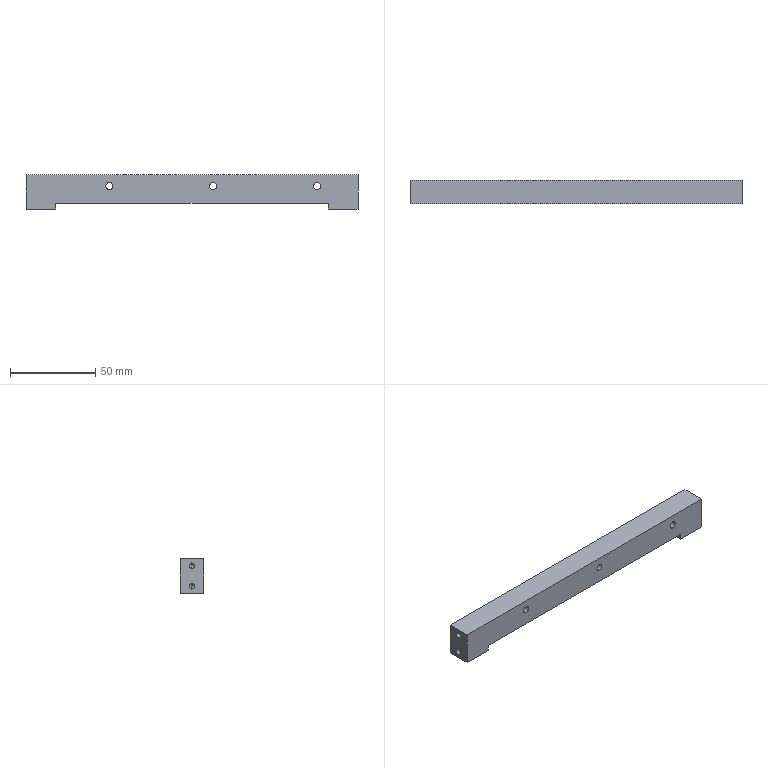Part | SolidWorks | features HoleWzd 3, ICE 2, ExtruThin 1 | 1 solid | 41 faces | box 195 x 14 x 20 mm | volume 45399 mm3 | cylinder 20 | plane 13 | cone 8 | commonest cylinder face diameters 3.3 x8 4.2 x6 8.8 x6
STEP:
#1=CARTESIAN_POINT('',(-19.6,11.,3.5));
#2=VERTEX_POINT('',#1);
#3=CARTESIAN_POINT('',(-28.4,11.,3.5));
#4=VERTEX_POINT('',#3);
#5=CARTESIAN_POINT('',(-24.,11.,3.5));
#6=DIRECTION('',(0.,1.,0.));
#7=DIRECTION('',(-1.,0.,0.));
#8=AXIS2_PLACEMENT_3D('',#5,#6,#7);
#9=CIRCLE('',#8,4.4);
#10=EDGE_CURVE('',#2,#4,#9,.T.);
#11=ORIENTED_EDGE('',*,*,#10,.F.);
#12=CARTESIAN_POINT('',(-19.6,14.,3.5));
#13=VERTEX_POINT('',#12);
#14=CARTESIAN_POINT('',(-19.6,11.,3.5));
#15=DIRECTION('',(0.,1.,0.));
#16=VECTOR('',#15,1000.);
#17=LINE('',#14,#16);
#18=EDGE_CURVE('',#2,#13,#17,.T.);
#19=ORIENTED_EDGE('',*,*,#18,.T.);
#20=CARTESIAN_POINT('',(-28.4,14.,3.5));
#21=VERTEX_POINT('',#20);
#22=CARTESIAN_POINT('',(-24.,14.,3.5));
#23=DIRECTION('',(0.,1.,0.));
#24=DIRECTION('',(-1.,0.,0.));
#25=AXIS2_PLACEMENT_3D('',#22,#23,#24);
#26=CIRCLE('',#25,4.4);
#27=EDGE_CURVE('',#13,#21,#26,.T.);
#28=ORIENTED_EDGE('',*,*,#27,.T.);
#29=CARTESIAN_POINT('',(-28.4,11.,3.5));
#30=DIRECTION('',(0.,1.,0.));
#31=VECTOR('',#30,1000.);
#32=LINE('',#29,#31);
#33=EDGE_CURVE('',#4,#21,#32,.T.);
#34=ORIENTED_EDGE('',*,*,#33,.F.);
#35=EDGE_LOOP('',(#11,#19,#28,#34));
#36=FACE_OUTER_BOUND('',#35,.T.);
#37=CARTESIAN_POINT('',(-24.,11.,3.5));
#38=DIRECTION('',(0.,1.,0.));
#39=DIRECTION('',(-1.,0.,0.));
#40=AXIS2_PLACEMENT_3D('',#37,#38,#39);
#41=CYLINDRICAL_SURFACE('',#40,4.4);
#42=ADVANCED_FACE('',(#36),#41,.F.);
#43=CARTESIAN_POINT('',(-80.6,11.,3.5));
#44=VERTEX_POINT('',#43);
#45=CARTESIAN_POINT('',(-89.4,11.,3.5));
#46=VERTEX_POINT('',#45);
#47=CARTESIAN_POINT('',(-85.,11.,3.5));
#48=DIRECTION('',(0.,1.,0.));
#49=DIRECTION('',(-1.,0.,0.));
#50=AXIS2_PLACEMENT_3D('',#47,#48,#49);
#51=CIRCLE('',#50,4.4);
#52=EDGE_CURVE('',#44,#46,#51,.T.);
#53=ORIENTED_EDGE('',*,*,#52,.F.);
#54=CARTESIAN_POINT('',(-80.6,14.,3.5));
#55=VERTEX_POINT('',#54);
#56=CARTESIAN_POINT('',(-80.6,11.,3.5));
#57=DIRECTION('',(0.,1.,0.));
#58=VECTOR('',#57,1000.);
#59=LINE('',#56,#58);
#60=EDGE_CURVE('',#44,#55,#59,.T.);
#61=ORIENTED_EDGE('',*,*,#60,.T.);
#62=CARTESIAN_POINT('',(-89.4,14.,3.5));
#63=VERTEX_POINT('',#62);
#64=CARTESIAN_POINT('',(-85.,14.,3.5));
#65=DIRECTION('',(0.,1.,0.));
#66=DIRECTION('',(-1.,0.,0.));
#67=AXIS2_PLACEMENT_3D('',#64,#65,#66);
#68=CIRCLE('',#67,4.4);
#69=EDGE_CURVE('',#55,#63,#68,.T.);
#70=ORIENTED_EDGE('',*,*,#69,.T.);
#71=CARTESIAN_POINT('',(-89.4,11.,3.5));
#72=DIRECTION('',(0.,1.,0.));
#73=VECTOR('',#72,1000.);
#74=LINE('',#71,#73);
#75=EDGE_CURVE('',#46,#63,#74,.T.);
#76=ORIENTED_EDGE('',*,*,#75,.F.);
#77=EDGE_LOOP('',(#53,#61,#70,#76));
#78=FACE_OUTER_BOUND('',#77,.T.);
#79=CARTESIAN_POINT('',(-85.,11.,3.5));
#80=DIRECTION('',(0.,1.,0.));
#81=DIRECTION('',(-1.,0.,0.));
#82=AXIS2_PLACEMENT_3D('',#79,#80,#81);
#83=CYLINDRICAL_SURFACE('',#82,4.4);
#84=ADVANCED_FACE('',(#78),#83,.F.);
#85=CARTESIAN_POINT('',(-141.6,11.,3.5));
#86=VERTEX_POINT('',#85);
#87=CARTESIAN_POINT('',(-150.4,11.,3.5));
#88=VERTEX_POINT('',#87);
#89=CARTESIAN_POINT('',(-146.,11.,3.5));
#90=DIRECTION('',(0.,1.,0.));
#91=DIRECTION('',(-1.,0.,0.));
#92=AXIS2_PLACEMENT_3D('',#89,#90,#91);
#93=CIRCLE('',#92,4.4);
#94=EDGE_CURVE('',#86,#88,#93,.T.);
#95=ORIENTED_EDGE('',*,*,#94,.F.);
#96=CARTESIAN_POINT('',(-141.6,14.,3.5));
#97=VERTEX_POINT('',#96);
#98=CARTESIAN_POINT('',(-141.6,11.,3.5));
#99=DIRECTION('',(0.,1.,0.));
#100=VECTOR('',#99,1000.);
#101=LINE('',#98,#100);
#102=EDGE_CURVE('',#86,#97,#101,.T.);
#103=ORIENTED_EDGE('',*,*,#102,.T.);
#104=CARTESIAN_POINT('',(-150.4,14.,3.5));
#105=VERTEX_POINT('',#104);
#106=CARTESIAN_POINT('',(-146.,14.,3.5));
#107=DIRECTION('',(0.,1.,0.));
#108=DIRECTION('',(-1.,0.,0.));
#109=AXIS2_PLACEMENT_3D('',#106,#107,#108);
#110=CIRCLE('',#109,4.4);
#111=EDGE_CURVE('',#97,#105,#110,.T.);
#112=ORIENTED_EDGE('',*,*,#111,.T.);
#113=CARTESIAN_POINT('',(-150.4,11.,3.5));
#114=DIRECTION('',(0.,1.,0.));
#115=VECTOR('',#114,1000.);
#116=LINE('',#113,#115);
#117=EDGE_CURVE('',#88,#105,#116,.T.);
#118=ORIENTED_EDGE('',*,*,#117,.F.);
#119=EDGE_LOOP('',(#95,#103,#112,#118));
#120=FACE_OUTER_BOUND('',#119,.T.);
#121=CARTESIAN_POINT('',(-146.,11.,3.5));
#122=DIRECTION('',(0.,1.,0.));
#123=DIRECTION('',(-1.,0.,0.));
#124=AXIS2_PLACEMENT_3D('',#121,#122,#123);
#125=CYLINDRICAL_SURFACE('',#124,4.4);
#126=ADVANCED_FACE('',(#120),#125,.F.);
#127=CARTESIAN_POINT('',(-10.1,7.,7.65));
#128=VERTEX_POINT('',#127);
#129=CARTESIAN_POINT('',(-10.1,7.,4.35));
#130=VERTEX_POINT('',#129);
#131=CARTESIAN_POINT('',(-10.1,7.,6.));
#132=DIRECTION('',(1.,0.,0.));
#133=DIRECTION('',(0.,0.,-1.));
#134=AXIS2_PLACEMENT_3D('',#131,#132,#133);
#135=CIRCLE('',#134,1.65);
#136=EDGE_CURVE('',#128,#130,#135,.T.);
#137=ORIENTED_EDGE('',*,*,#136,.F.);
#138=CARTESIAN_POINT('',(0.,7.,7.65));
#139=VERTEX_POINT('',#138);
#140=CARTESIAN_POINT('',(0.,7.,7.65));
#141=DIRECTION('',(1.,0.,0.));
#142=VECTOR('',#141,1000.);
#143=LINE('',#140,#142);
#144=EDGE_CURVE('',#128,#139,#143,.T.);
#145=ORIENTED_EDGE('',*,*,#144,.T.);
#146=CARTESIAN_POINT('',(0.,7.,4.35));
#147=VERTEX_POINT('',#146);
#148=CARTESIAN_POINT('',(0.,7.,6.));
#149=DIRECTION('',(1.,0.,0.));
#150=DIRECTION('',(0.,0.,-1.));
#151=AXIS2_PLACEMENT_3D('',#148,#149,#150);
#152=CIRCLE('',#151,1.65);
#153=EDGE_CURVE('',#139,#147,#152,.T.);
#154=ORIENTED_EDGE('',*,*,#153,.T.);
#155=CARTESIAN_POINT('',(0.,7.,4.35));
#156=DIRECTION('',(1.,0.,0.));
#157=VECTOR('',#156,1000.);
#158=LINE('',#155,#157);
#159=EDGE_CURVE('',#130,#147,#158,.T.);
#160=ORIENTED_EDGE('',*,*,#159,.F.);
#161=EDGE_LOOP('',(#137,#145,#154,#160));
#162=FACE_OUTER_BOUND('',#161,.T.);
#163=CARTESIAN_POINT('',(0.,7.,6.));
#164=DIRECTION('',(1.,0.,0.));
#165=DIRECTION('',(0.,0.,-1.));
#166=AXIS2_PLACEMENT_3D('',#163,#164,#165);
#167=CYLINDRICAL_SURFACE('',#166,1.65);
#168=ADVANCED_FACE('',(#162),#167,.F.);
#169=CARTESIAN_POINT('',(-11.091,7.,6.));
#170=VERTEX_POINT('',#169);
#171=CARTESIAN_POINT('',(-10.1,7.,4.35));
#172=DIRECTION('',(0.515,0.,-0.8572));
#173=VECTOR('',#172,1000.);
#174=LINE('',#171,#173);
#175=EDGE_CURVE('',#170,#130,#174,.T.);
#176=ORIENTED_EDGE('',*,*,#175,.F.);
#177=CARTESIAN_POINT('',(-10.1,7.,7.65));
#178=DIRECTION('',(0.515,0.,0.8572));
#179=VECTOR('',#178,1000.);
#180=LINE('',#177,#179);
#181=EDGE_CURVE('',#170,#128,#180,.T.);
#182=ORIENTED_EDGE('',*,*,#181,.T.);
#183=ORIENTED_EDGE('',*,*,#136,.T.);
#184=EDGE_LOOP('',(#176,#182,#183));
#185=FACE_OUTER_BOUND('',#184,.T.);
#186=CARTESIAN_POINT('',(-10.1,7.,6.));
#187=DIRECTION('',(1.,0.,0.));
#188=DIRECTION('',(0.,0.,-1.));
#189=AXIS2_PLACEMENT_3D('',#186,#187,#188);
#190=CONICAL_SURFACE('',#189,1.65,1.03);
#191=ADVANCED_FACE('',(#185),#190,.F.);
#192=CARTESIAN_POINT('',(-10.1,7.,-4.35));
#193=VERTEX_POINT('',#192);
#194=CARTESIAN_POINT('',(-10.1,7.,-7.65));
#195=VERTEX_POINT('',#194);
#196=CARTESIAN_POINT('',(-10.1,7.,-6.));
#197=DIRECTION('',(1.,0.,0.));
#198=DIRECTION('',(0.,0.,-1.));
#199=AXIS2_PLACEMENT_3D('',#196,#197,#198);
#200=CIRCLE('',#199,1.65);
#201=EDGE_CURVE('',#193,#195,#200,.T.);
#202=ORIENTED_EDGE('',*,*,#201,.F.);
#203=CARTESIAN_POINT('',(0.,7.,-4.35));
#204=VERTEX_POINT('',#203);
#205=CARTESIAN_POINT('',(0.,7.,-4.35));
#206=DIRECTION('',(1.,0.,0.));
#207=VECTOR('',#206,1000.);
#208=LINE('',#205,#207);
#209=EDGE_CURVE('',#193,#204,#208,.T.);
#210=ORIENTED_EDGE('',*,*,#209,.T.);
#211=CARTESIAN_POINT('',(0.,7.,-7.65));
#212=VERTEX_POINT('',#211);
#213=CARTESIAN_POINT('',(0.,7.,-6.));
#214=DIRECTION('',(1.,0.,0.));
#215=DIRECTION('',(0.,0.,-1.));
#216=AXIS2_PLACEMENT_3D('',#213,#214,#215);
#217=CIRCLE('',#216,1.65);
#218=EDGE_CURVE('',#204,#212,#217,.T.);
#219=ORIENTED_EDGE('',*,*,#218,.T.);
#220=CARTESIAN_POINT('',(0.,7.,-7.65));
#221=DIRECTION('',(1.,0.,0.));
#222=VECTOR('',#221,1000.);
#223=LINE('',#220,#222);
#224=EDGE_CURVE('',#195,#212,#223,.T.);
#225=ORIENTED_EDGE('',*,*,#224,.F.);
#226=EDGE_LOOP('',(#202,#210,#219,#225));
#227=FACE_OUTER_BOUND('',#226,.T.);
#228=CARTESIAN_POINT('',(0.,7.,-6.));
#229=DIRECTION('',(1.,0.,0.));
#230=DIRECTION('',(0.,0.,-1.));
#231=AXIS2_PLACEMENT_3D('',#228,#229,#230);
#232=CYLINDRICAL_SURFACE('',#231,1.65);
#233=ADVANCED_FACE('',(#227),#232,.F.);
#234=CARTESIAN_POINT('',(-11.091,7.,-6.));
#235=VERTEX_POINT('',#234);
#236=CARTESIAN_POINT('',(-10.1,7.,-7.65));
#237=DIRECTION('',(0.515,0.,-0.8572));
#238=VECTOR('',#237,1000.);
#239=LINE('',#236,#238);
#240=EDGE_CURVE('',#235,#195,#239,.T.);
#241=ORIENTED_EDGE('',*,*,#240,.F.);
#242=CARTESIAN_POINT('',(-10.1,7.,-4.35));
#243=DIRECTION('',(0.515,0.,0.8572));
#244=VECTOR('',#243,1000.);
#245=LINE('',#242,#244);
#246=EDGE_CURVE('',#235,#193,#245,.T.);
#247=ORIENTED_EDGE('',*,*,#246,.T.);
#248=ORIENTED_EDGE('',*,*,#201,.T.);
#249=EDGE_LOOP('',(#241,#247,#248));
#250=FACE_OUTER_BOUND('',#249,.T.);
#251=CARTESIAN_POINT('',(-10.1,7.,-6.));
#252=DIRECTION('',(1.,0.,0.));
#253=DIRECTION('',(0.,0.,-1.));
#254=AXIS2_PLACEMENT_3D('',#251,#252,#253);
#255=CONICAL_SURFACE('',#254,1.65,1.03);
#256=ADVANCED_FACE('',(#250),#255,.F.);
#257=CARTESIAN_POINT('',(-184.9,7.,-7.65));
#258=VERTEX_POINT('',#257);
#259=CARTESIAN_POINT('',(-184.9,7.,-4.35));
#260=VERTEX_POINT('',#259);
#261=CARTESIAN_POINT('',(-184.9,7.,-6.));
#262=DIRECTION('',(-1.,0.,0.));
#263=DIRECTION('',(0.,0.,1.));
#264=AXIS2_PLACEMENT_3D('',#261,#262,#263);
#265=CIRCLE('',#264,1.65);
#266=EDGE_CURVE('',#258,#260,#265,.T.);
#267=ORIENTED_EDGE('',*,*,#266,.F.);
#268=CARTESIAN_POINT('',(-195.,7.,-7.65));
#269=VERTEX_POINT('',#268);
#270=CARTESIAN_POINT('',(-195.,7.,-7.65));
#271=DIRECTION('',(-1.,0.,0.));
#272=VECTOR('',#271,1000.);
#273=LINE('',#270,#272);
#274=EDGE_CURVE('',#258,#269,#273,.T.);
#275=ORIENTED_EDGE('',*,*,#274,.T.);
#276=CARTESIAN_POINT('',(-195.,7.,-4.35));
#277=VERTEX_POINT('',#276);
#278=CARTESIAN_POINT('',(-195.,7.,-6.));
#279=DIRECTION('',(-1.,0.,0.));
#280=DIRECTION('',(0.,0.,1.));
#281=AXIS2_PLACEMENT_3D('',#278,#279,#280);
#282=CIRCLE('',#281,1.65);
#283=EDGE_CURVE('',#269,#277,#282,.T.);
#284=ORIENTED_EDGE('',*,*,#283,.T.);
#285=CARTESIAN_POINT('',(-195.,7.,-4.35));
#286=DIRECTION('',(-1.,0.,0.));
#287=VECTOR('',#286,1000.);
#288=LINE('',#285,#287);
#289=EDGE_CURVE('',#260,#277,#288,.T.);
#290=ORIENTED_EDGE('',*,*,#289,.F.);
#291=EDGE_LOOP('',(#267,#275,#284,#290));
#292=FACE_OUTER_BOUND('',#291,.T.);
#293=CARTESIAN_POINT('',(-195.,7.,-6.));
#294=DIRECTION('',(-1.,0.,0.));
#295=DIRECTION('',(0.,0.,1.));
#296=AXIS2_PLACEMENT_3D('',#293,#294,#295);
#297=CYLINDRICAL_SURFACE('',#296,1.65);
#298=ADVANCED_FACE('',(#292),#297,.F.);
#299=CARTESIAN_POINT('',(-183.909,7.,-6.));
#300=VERTEX_POINT('',#299);
#301=CARTESIAN_POINT('',(-184.9,7.,-4.35));
#302=DIRECTION('',(-0.515,0.,0.8572));
#303=VECTOR('',#302,1000.);
#304=LINE('',#301,#303);
#305=EDGE_CURVE('',#300,#260,#304,.T.);
#306=ORIENTED_EDGE('',*,*,#305,.F.);
#307=CARTESIAN_POINT('',(-184.9,7.,-7.65));
#308=DIRECTION('',(-0.515,0.,-0.8572));
#309=VECTOR('',#308,1000.);
#310=LINE('',#307,#309);
#311=EDGE_CURVE('',#300,#258,#310,.T.);
#312=ORIENTED_EDGE('',*,*,#311,.T.);
#313=ORIENTED_EDGE('',*,*,#266,.T.);
#314=EDGE_LOOP('',(#306,#312,#313));
#315=FACE_OUTER_BOUND('',#314,.T.);
#316=CARTESIAN_POINT('',(-184.9,7.,-6.));
#317=DIRECTION('',(-1.,0.,0.));
#318=DIRECTION('',(0.,0.,1.));
#319=AXIS2_PLACEMENT_3D('',#316,#317,#318);
#320=CONICAL_SURFACE('',#319,1.65,1.03);
#321=ADVANCED_FACE('',(#315),#320,.F.);
#322=CARTESIAN_POINT('',(-184.9,7.,4.35));
#323=VERTEX_POINT('',#322);
#324=CARTESIAN_POINT('',(-184.9,7.,7.65));
#325=VERTEX_POINT('',#324);
#326=CARTESIAN_POINT('',(-184.9,7.,6.));
#327=DIRECTION('',(-1.,0.,0.));
#328=DIRECTION('',(0.,0.,1.));
#329=AXIS2_PLACEMENT_3D('',#326,#327,#328);
#330=CIRCLE('',#329,1.65);
#331=EDGE_CURVE('',#323,#325,#330,.T.);
#332=ORIENTED_EDGE('',*,*,#331,.F.);
#333=CARTESIAN_POINT('',(-195.,7.,4.35));
#334=VERTEX_POINT('',#333);
#335=CARTESIAN_POINT('',(-195.,7.,4.35));
#336=DIRECTION('',(-1.,0.,0.));
#337=VECTOR('',#336,1000.);
#338=LINE('',#335,#337);
#339=EDGE_CURVE('',#323,#334,#338,.T.);
#340=ORIENTED_EDGE('',*,*,#339,.T.);
#341=CARTESIAN_POINT('',(-195.,7.,7.65));
#342=VERTEX_POINT('',#341);
#343=CARTESIAN_POINT('',(-195.,7.,6.));
#344=DIRECTION('',(-1.,0.,0.));
#345=DIRECTION('',(0.,0.,1.));
#346=AXIS2_PLACEMENT_3D('',#343,#344,#345);
#347=CIRCLE('',#346,1.65);
#348=EDGE_CURVE('',#334,#342,#347,.T.);
#349=ORIENTED_EDGE('',*,*,#348,.T.);
#350=CARTESIAN_POINT('',(-195.,7.,7.65));
#351=DIRECTION('',(-1.,0.,0.));
#352=VECTOR('',#351,1000.);
#353=LINE('',#350,#352);
#354=EDGE_CURVE('',#325,#342,#353,.T.);
#355=ORIENTED_EDGE('',*,*,#354,.F.);
#356=EDGE_LOOP('',(#332,#340,#349,#355));
#357=FACE_OUTER_BOUND('',#356,.T.);
#358=CARTESIAN_POINT('',(-195.,7.,6.));
#359=DIRECTION('',(-1.,0.,0.));
#360=DIRECTION('',(0.,0.,1.));
#361=AXIS2_PLACEMENT_3D('',#358,#359,#360);
#362=CYLINDRICAL_SURFACE('',#361,1.65);
#363=ADVANCED_FACE('',(#357),#362,.F.);
#364=CARTESIAN_POINT('',(-183.909,7.,6.));
#365=VERTEX_POINT('',#364);
#366=CARTESIAN_POINT('',(-184.9,7.,7.65));
#367=DIRECTION('',(-0.515,0.,0.8572));
#368=VECTOR('',#367,1000.);
#369=LINE('',#366,#368);
#370=EDGE_CURVE('',#365,#325,#369,.T.);
#371=ORIENTED_EDGE('',*,*,#370,.F.);
#372=CARTESIAN_POINT('',(-184.9,7.,4.35));
#373=DIRECTION('',(-0.515,0.,-0.8572));
#374=VECTOR('',#373,1000.);
#375=LINE('',#372,#374);
#376=EDGE_CURVE('',#365,#323,#375,.T.);
#377=ORIENTED_EDGE('',*,*,#376,.T.);
#378=ORIENTED_EDGE('',*,*,#331,.T.);
#379=EDGE_LOOP('',(#371,#377,#378));
#380=FACE_OUTER_BOUND('',#379,.T.);
#381=CARTESIAN_POINT('',(-184.9,7.,6.));
#382=DIRECTION('',(-1.,0.,0.));
#383=DIRECTION('',(0.,0.,1.));
#384=AXIS2_PLACEMENT_3D('',#381,#382,#383);
#385=CONICAL_SURFACE('',#384,1.65,1.03);
#386=ADVANCED_FACE('',(#380),#385,.F.);
#387=CARTESIAN_POINT('',(-146.,0.,1.4));
#388=VERTEX_POINT('',#387);
#389=CARTESIAN_POINT('',(-146.,0.,5.6));
#390=VERTEX_POINT('',#389);
#391=CARTESIAN_POINT('',(-146.,0.,3.5));
#392=DIRECTION('',(0.,1.,0.));
#393=DIRECTION('',(0.,0.,1.));
#394=AXIS2_PLACEMENT_3D('',#391,#392,#393);
#395=CIRCLE('',#394,2.1);
#396=EDGE_CURVE('',#388,#390,#395,.T.);
#397=ORIENTED_EDGE('',*,*,#396,.F.);
#398=CARTESIAN_POINT('',(-146.,11.,1.4));
#399=VERTEX_POINT('',#398);
#400=CARTESIAN_POINT('',(-146.,14.,1.4));
#401=DIRECTION('',(0.,1.,0.));
#402=VECTOR('',#401,1000.);
#403=LINE('',#400,#402);
#404=EDGE_CURVE('',#388,#399,#403,.T.);
#405=ORIENTED_EDGE('',*,*,#404,.T.);
#406=CARTESIAN_POINT('',(-146.,11.,5.6));
#407=VERTEX_POINT('',#406);
#408=CARTESIAN_POINT('',(-146.,11.,3.5));
#409=DIRECTION('',(0.,-1.,0.));
#410=DIRECTION('',(-1.,0.,0.));
#411=AXIS2_PLACEMENT_3D('',#408,#409,#410);
#412=CIRCLE('',#411,2.1);
#413=EDGE_CURVE('',#407,#399,#412,.T.);
#414=ORIENTED_EDGE('',*,*,#413,.F.);
#415=CARTESIAN_POINT('',(-146.,14.,5.6));
#416=DIRECTION('',(0.,1.,0.));
#417=VECTOR('',#416,1000.);
#418=LINE('',#415,#417);
#419=EDGE_CURVE('',#390,#407,#418,.T.);
#420=ORIENTED_EDGE('',*,*,#419,.F.);
#421=EDGE_LOOP('',(#397,#405,#414,#420));
#422=FACE_OUTER_BOUND('',#421,.T.);
#423=CARTESIAN_POINT('',(-146.,14.,3.5));
#424=DIRECTION('',(0.,1.,0.));
#425=DIRECTION('',(0.,0.,1.));
#426=AXIS2_PLACEMENT_3D('',#423,#424,#425);
#427=CYLINDRICAL_SURFACE('',#426,2.1);
#428=ADVANCED_FACE('',(#422),#427,.F.);
#429=CARTESIAN_POINT('',(-85.,0.,1.4));
#430=VERTEX_POINT('',#429);
#431=CARTESIAN_POINT('',(-85.,0.,5.6));
#432=VERTEX_POINT('',#431);
#433=CARTESIAN_POINT('',(-85.,0.,3.5));
#434=DIRECTION('',(0.,1.,0.));
#435=DIRECTION('',(0.,0.,1.));
#436=AXIS2_PLACEMENT_3D('',#433,#434,#435);
#437=CIRCLE('',#436,2.1);
#438=EDGE_CURVE('',#430,#432,#437,.T.);
#439=ORIENTED_EDGE('',*,*,#438,.F.);
#440=CARTESIAN_POINT('',(-85.,11.,1.4));
#441=VERTEX_POINT('',#440);
#442=CARTESIAN_POINT('',(-85.,14.,1.4));
#443=DIRECTION('',(0.,1.,0.));
#444=VECTOR('',#443,1000.);
#445=LINE('',#442,#444);
#446=EDGE_CURVE('',#430,#441,#445,.T.);
#447=ORIENTED_EDGE('',*,*,#446,.T.);
#448=CARTESIAN_POINT('',(-85.,11.,5.6));
#449=VERTEX_POINT('',#448);
#450=CARTESIAN_POINT('',(-85.,11.,3.5));
#451=DIRECTION('',(0.,-1.,0.));
#452=DIRECTION('',(-1.,0.,0.));
#453=AXIS2_PLACEMENT_3D('',#450,#451,#452);
#454=CIRCLE('',#453,2.1);
#455=EDGE_CURVE('',#449,#441,#454,.T.);
#456=ORIENTED_EDGE('',*,*,#455,.F.);
#457=CARTESIAN_POINT('',(-85.,14.,5.6));
#458=DIRECTION('',(0.,1.,0.));
#459=VECTOR('',#458,1000.);
#460=LINE('',#457,#459);
#461=EDGE_CURVE('',#432,#449,#460,.T.);
#462=ORIENTED_EDGE('',*,*,#461,.F.);
#463=EDGE_LOOP('',(#439,#447,#456,#462));
#464=FACE_OUTER_BOUND('',#463,.T.);
#465=CARTESIAN_POINT('',(-85.,14.,3.5));
#466=DIRECTION('',(0.,1.,0.));
#467=DIRECTION('',(0.,0.,1.));
#468=AXIS2_PLACEMENT_3D('',#465,#466,#467);
#469=CYLINDRICAL_SURFACE('',#468,2.1);
#470=ADVANCED_FACE('',(#464),#469,.F.);
#471=CARTESIAN_POINT('',(-24.,0.,1.4));
#472=VERTEX_POINT('',#471);
#473=CARTESIAN_POINT('',(-24.,0.,5.6));
#474=VERTEX_POINT('',#473);
#475=CARTESIAN_POINT('',(-24.,0.,3.5));
#476=DIRECTION('',(0.,1.,0.));
#477=DIRECTION('',(0.,0.,1.));
#478=AXIS2_PLACEMENT_3D('',#475,#476,#477);
#479=CIRCLE('',#478,2.1);
#480=EDGE_CURVE('',#472,#474,#479,.T.);
#481=ORIENTED_EDGE('',*,*,#480,.F.);
#482=CARTESIAN_POINT('',(-24.,11.,1.4));
#483=VERTEX_POINT('',#482);
#484=CARTESIAN_POINT('',(-24.,14.,1.4));
#485=DIRECTION('',(0.,1.,0.));
#486=VECTOR('',#485,1000.);
#487=LINE('',#484,#486);
#488=EDGE_CURVE('',#472,#483,#487,.T.);
#489=ORIENTED_EDGE('',*,*,#488,.T.);
#490=CARTESIAN_POINT('',(-24.,11.,5.6));
#491=VERTEX_POINT('',#490);
#492=CARTESIAN_POINT('',(-24.,11.,3.5));
#493=DIRECTION('',(0.,-1.,0.));
#494=DIRECTION('',(-1.,0.,0.));
#495=AXIS2_PLACEMENT_3D('',#492,#493,#494);
#496=CIRCLE('',#495,2.1);
#497=EDGE_CURVE('',#491,#483,#496,.T.);
#498=ORIENTED_EDGE('',*,*,#497,.F.);
#499=CARTESIAN_POINT('',(-24.,14.,5.6));
#500=DIRECTION('',(0.,1.,0.));
#501=VECTOR('',#500,1000.);
#502=LINE('',#499,#501);
#503=EDGE_CURVE('',#474,#491,#502,.T.);
#504=ORIENTED_EDGE('',*,*,#503,.F.);
#505=EDGE_LOOP('',(#481,#489,#498,#504));
#506=FACE_OUTER_BOUND('',#505,.T.);
#507=CARTESIAN_POINT('',(-24.,14.,3.5));
#508=DIRECTION('',(0.,1.,0.));
#509=DIRECTION('',(0.,0.,1.));
#510=AXIS2_PLACEMENT_3D('',#507,#508,#509);
#511=CYLINDRICAL_SURFACE('',#510,2.1);
#512=ADVANCED_FACE('',(#506),#511,.F.);
#513=CARTESIAN_POINT('',(-177.5,0.,-10.));
#514=VERTEX_POINT('',#513);
#515=CARTESIAN_POINT('',(-177.5,14.,-10.));
#516=VERTEX_POINT('',#515);
#517=CARTESIAN_POINT('',(-177.5,0.,-10.));
#518=DIRECTION('',(0.,1.,0.));
#519=VECTOR('',#518,1000.);
#520=LINE('',#517,#519);
#521=EDGE_CURVE('',#514,#516,#520,.T.);
#522=ORIENTED_EDGE('',*,*,#521,.F.);
#523=CARTESIAN_POINT('',(-195.,0.,-10.));
#524=VERTEX_POINT('',#523);
#525=CARTESIAN_POINT('',(0.,0.,-10.));
#526=DIRECTION('',(-1.,0.,0.));
#527=VECTOR('',#526,1000.);
#528=LINE('',#525,#527);
#529=EDGE_CURVE('',#514,#524,#528,.T.);
#530=ORIENTED_EDGE('',*,*,#529,.T.);
#531=CARTESIAN_POINT('',(-195.,14.,-10.));
#532=VERTEX_POINT('',#531);
#533=CARTESIAN_POINT('',(-195.,0.,-10.));
#534=DIRECTION('',(0.,1.,0.));
#535=VECTOR('',#534,1000.);
#536=LINE('',#533,#535);
#537=EDGE_CURVE('',#524,#532,#536,.T.);
#538=ORIENTED_EDGE('',*,*,#537,.T.);
#539=CARTESIAN_POINT('',(0.,14.,-10.));
#540=DIRECTION('',(-1.,0.,0.));
#541=VECTOR('',#540,1000.);
#542=LINE('',#539,#541);
#543=EDGE_CURVE('',#516,#532,#542,.T.);
#544=ORIENTED_EDGE('',*,*,#543,.F.);
#545=EDGE_LOOP('',(#522,#530,#538,#544));
#546=FACE_OUTER_BOUND('',#545,.T.);
#547=CARTESIAN_POINT('',(0.,0.,-10.));
#548=DIRECTION('',(0.,0.,-1.));
#549=DIRECTION('',(-1.,0.,0.));
#550=AXIS2_PLACEMENT_3D('',#547,#548,#549);
#551=PLANE('',#550);
#552=ADVANCED_FACE('',(#546),#551,.T.);
#553=ORIENTED_EDGE('',*,*,#488,.F.);
#554=CARTESIAN_POINT('',(-24.,0.,3.5));
#555=DIRECTION('',(0.,1.,0.));
#556=DIRECTION('',(0.,0.,1.));
#557=AXIS2_PLACEMENT_3D('',#554,#555,#556);
#558=CIRCLE('',#557,2.1);
#559=EDGE_CURVE('',#474,#472,#558,.T.);
#560=ORIENTED_EDGE('',*,*,#559,.F.);
#561=ORIENTED_EDGE('',*,*,#503,.T.);
#562=CARTESIAN_POINT('',(-24.,11.,3.5));
#563=DIRECTION('',(0.,-1.,0.));
#564=DIRECTION('',(-1.,0.,0.));
#565=AXIS2_PLACEMENT_3D('',#562,#563,#564);
#566=CIRCLE('',#565,2.1);
#567=EDGE_CURVE('',#483,#491,#566,.T.);
#568=ORIENTED_EDGE('',*,*,#567,.F.);
#569=EDGE_LOOP('',(#553,#560,#561,#568));
#570=FACE_OUTER_BOUND('',#569,.T.);
#571=CARTESIAN_POINT('',(-24.,14.,3.5));
#572=DIRECTION('',(0.,1.,0.));
#573=DIRECTION('',(0.,0.,1.));
#574=AXIS2_PLACEMENT_3D('',#571,#572,#573);
#575=CYLINDRICAL_SURFACE('',#574,2.1);
#576=ADVANCED_FACE('',(#570),#575,.F.);
#577=ORIENTED_EDGE('',*,*,#446,.F.);
#578=CARTESIAN_POINT('',(-85.,0.,3.5));
#579=DIRECTION('',(0.,1.,0.));
#580=DIRECTION('',(0.,0.,1.));
#581=AXIS2_PLACEMENT_3D('',#578,#579,#580);
#582=CIRCLE('',#581,2.1);
#583=EDGE_CURVE('',#432,#430,#582,.T.);
#584=ORIENTED_EDGE('',*,*,#583,.F.);
#585=ORIENTED_EDGE('',*,*,#461,.T.);
#586=CARTESIAN_POINT('',(-85.,11.,3.5));
#587=DIRECTION('',(0.,-1.,0.));
#588=DIRECTION('',(-1.,0.,0.));
#589=AXIS2_PLACEMENT_3D('',#586,#587,#588);
#590=CIRCLE('',#589,2.1);
#591=EDGE_CURVE('',#441,#449,#590,.T.);
#592=ORIENTED_EDGE('',*,*,#591,.F.);
#593=EDGE_LOOP('',(#577,#584,#585,#592));
#594=FACE_OUTER_BOUND('',#593,.T.);
#595=CARTESIAN_POINT('',(-85.,14.,3.5));
#596=DIRECTION('',(0.,1.,0.));
#597=DIRECTION('',(0.,0.,1.));
#598=AXIS2_PLACEMENT_3D('',#595,#596,#597);
#599=CYLINDRICAL_SURFACE('',#598,2.1);
#600=ADVANCED_FACE('',(#594),#599,.F.);
#601=ORIENTED_EDGE('',*,*,#404,.F.);
#602=CARTESIAN_POINT('',(-146.,0.,3.5));
#603=DIRECTION('',(0.,1.,0.));
#604=DIRECTION('',(0.,0.,1.));
#605=AXIS2_PLACEMENT_3D('',#602,#603,#604);
#606=CIRCLE('',#605,2.1);
#607=EDGE_CURVE('',#390,#388,#606,.T.);
#608=ORIENTED_EDGE('',*,*,#607,.F.);
#609=ORIENTED_EDGE('',*,*,#419,.T.);
#610=CARTESIAN_POINT('',(-146.,11.,3.5));
#611=DIRECTION('',(0.,-1.,0.));
#612=DIRECTION('',(-1.,0.,0.));
#613=AXIS2_PLACEMENT_3D('',#610,#611,#612);
#614=CIRCLE('',#613,2.1);
#615=EDGE_CURVE('',#399,#407,#614,.T.);
#616=ORIENTED_EDGE('',*,*,#615,.F.);
#617=EDGE_LOOP('',(#601,#608,#609,#616));
#618=FACE_OUTER_BOUND('',#617,.T.);
#619=CARTESIAN_POINT('',(-146.,14.,3.5));
#620=DIRECTION('',(0.,1.,0.));
#621=DIRECTION('',(0.,0.,1.));
#622=AXIS2_PLACEMENT_3D('',#619,#620,#621);
#623=CYLINDRICAL_SURFACE('',#622,2.1);
#624=ADVANCED_FACE('',(#618),#623,.F.);
#625=CARTESIAN_POINT('',(-146.,14.,3.5));
#626=DIRECTION('',(0.,1.,0.));
#627=DIRECTION('',(-1.,0.,0.));
#628=AXIS2_PLACEMENT_3D('',#625,#626,#627);
#629=CIRCLE('',#628,4.4);
#630=EDGE_CURVE('',#105,#97,#629,.T.);
#631=ORIENTED_EDGE('',*,*,#630,.F.);
#632=ORIENTED_EDGE('',*,*,#111,.F.);
#633=EDGE_LOOP('',(#631,#632));
#634=FACE_BOUND('',#633,.T.);
#635=CARTESIAN_POINT('',(-85.,14.,3.5));
#636=DIRECTION('',(0.,1.,0.));
#637=DIRECTION('',(-1.,0.,0.));
#638=AXIS2_PLACEMENT_3D('',#635,#636,#637);
#639=CIRCLE('',#638,4.4);
#640=EDGE_CURVE('',#63,#55,#639,.T.);
#641=ORIENTED_EDGE('',*,*,#640,.F.);
#642=ORIENTED_EDGE('',*,*,#69,.F.);
#643=EDGE_LOOP('',(#641,#642));
#644=FACE_BOUND('',#643,.T.);
#645=CARTESIAN_POINT('',(-24.,14.,3.5));
#646=DIRECTION('',(0.,1.,0.));
#647=DIRECTION('',(-1.,0.,0.));
#648=AXIS2_PLACEMENT_3D('',#645,#646,#647);
#649=CIRCLE('',#648,4.4);
#650=EDGE_CURVE('',#21,#13,#649,.T.);
#651=ORIENTED_EDGE('',*,*,#650,.F.);
#652=ORIENTED_EDGE('',*,*,#27,.F.);
#653=EDGE_LOOP('',(#651,#652));
#654=FACE_BOUND('',#653,.T.);
#655=CARTESIAN_POINT('',(-177.5,14.,-6.5));
#656=VERTEX_POINT('',#655);
#657=CARTESIAN_POINT('',(-17.5,14.,-6.5));
#658=VERTEX_POINT('',#657);
#659=CARTESIAN_POINT('',(-177.5,14.,-6.5));
#660=DIRECTION('',(1.,0.,0.));
#661=VECTOR('',#660,1000.);
#662=LINE('',#659,#661);
#663=EDGE_CURVE('',#656,#658,#662,.T.);
#664=ORIENTED_EDGE('',*,*,#663,.F.);
#665=CARTESIAN_POINT('',(-177.5,14.,-10.));
#666=DIRECTION('',(0.,0.,1.));
#667=VECTOR('',#666,1000.);
#668=LINE('',#665,#667);
#669=EDGE_CURVE('',#516,#656,#668,.T.);
#670=ORIENTED_EDGE('',*,*,#669,.F.);
#671=ORIENTED_EDGE('',*,*,#543,.T.);
#672=CARTESIAN_POINT('',(-195.,14.,10.));
#673=VERTEX_POINT('',#672);
#674=CARTESIAN_POINT('',(-195.,14.,10.));
#675=DIRECTION('',(0.,0.,-1.));
#676=VECTOR('',#675,1000.);
#677=LINE('',#674,#676);
#678=EDGE_CURVE('',#673,#532,#677,.T.);
#679=ORIENTED_EDGE('',*,*,#678,.F.);
#680=CARTESIAN_POINT('',(0.,14.,10.));
#681=VERTEX_POINT('',#680);
#682=CARTESIAN_POINT('',(0.,14.,10.));
#683=DIRECTION('',(-1.,0.,0.));
#684=VECTOR('',#683,1000.);
#685=LINE('',#682,#684);
#686=EDGE_CURVE('',#681,#673,#685,.T.);
#687=ORIENTED_EDGE('',*,*,#686,.F.);
#688=CARTESIAN_POINT('',(0.,14.,-10.));
#689=VERTEX_POINT('',#688);
#690=CARTESIAN_POINT('',(0.,14.,10.));
#691=DIRECTION('',(0.,0.,-1.));
#692=VECTOR('',#691,1000.);
#693=LINE('',#690,#692);
#694=EDGE_CURVE('',#681,#689,#693,.T.);
#695=ORIENTED_EDGE('',*,*,#694,.T.);
#696=CARTESIAN_POINT('',(-17.5,14.,-10.));
#697=VERTEX_POINT('',#696);
#698=CARTESIAN_POINT('',(0.,14.,-10.));
#699=DIRECTION('',(-1.,0.,0.));
#700=VECTOR('',#699,1000.);
#701=LINE('',#698,#700);
#702=EDGE_CURVE('',#689,#697,#701,.T.);
#703=ORIENTED_EDGE('',*,*,#702,.T.);
#704=CARTESIAN_POINT('',(-17.5,14.,-10.));
#705=DIRECTION('',(0.,0.,-1.));
#706=VECTOR('',#705,1000.);
#707=LINE('',#704,#706);
#708=EDGE_CURVE('',#658,#697,#707,.T.);
#709=ORIENTED_EDGE('',*,*,#708,.F.);
#710=EDGE_LOOP('',(#664,#670,#671,#679,#687,#695,#703,#709));
#711=FACE_OUTER_BOUND('',#710,.T.);
#712=CARTESIAN_POINT('',(0.,14.,10.));
#713=DIRECTION('',(0.,-1.,0.));
#714=DIRECTION('',(1.,0.,0.));
#715=AXIS2_PLACEMENT_3D('',#712,#713,#714);
#716=PLANE('',#715);
#717=ADVANCED_FACE('',(#634,#644,#654,#711),#716,.F.);
#718=CARTESIAN_POINT('',(-195.,7.,-6.));
#719=DIRECTION('',(-1.,0.,0.));
#720=DIRECTION('',(0.,0.,1.));
#721=AXIS2_PLACEMENT_3D('',#718,#719,#720);
#722=CIRCLE('',#721,1.65);
#723=EDGE_CURVE('',#277,#269,#722,.T.);
#724=ORIENTED_EDGE('',*,*,#723,.F.);
#725=ORIENTED_EDGE('',*,*,#283,.F.);
#726=EDGE_LOOP('',(#724,#725));
#727=FACE_BOUND('',#726,.T.);
#728=CARTESIAN_POINT('',(-195.,7.,6.));
#729=DIRECTION('',(-1.,0.,0.));
#730=DIRECTION('',(0.,0.,1.));
#731=AXIS2_PLACEMENT_3D('',#728,#729,#730);
#732=CIRCLE('',#731,1.65);
#733=EDGE_CURVE('',#342,#334,#732,.T.);
#734=ORIENTED_EDGE('',*,*,#733,.F.);
#735=ORIENTED_EDGE('',*,*,#348,.F.);
#736=EDGE_LOOP('',(#734,#735));
#737=FACE_BOUND('',#736,.T.);
#738=ORIENTED_EDGE('',*,*,#537,.F.);
#739=CARTESIAN_POINT('',(-195.,0.,10.));
#740=VERTEX_POINT('',#739);
#741=CARTESIAN_POINT('',(-195.,0.,10.));
#742=DIRECTION('',(0.,0.,-1.));
#743=VECTOR('',#742,1000.);
#744=LINE('',#741,#743);
#745=EDGE_CURVE('',#740,#524,#744,.T.);
#746=ORIENTED_EDGE('',*,*,#745,.F.);
#747=CARTESIAN_POINT('',(-195.,0.,10.));
#748=DIRECTION('',(0.,1.,0.));
#749=VECTOR('',#748,1000.);
#750=LINE('',#747,#749);
#751=EDGE_CURVE('',#740,#673,#750,.T.);
#752=ORIENTED_EDGE('',*,*,#751,.T.);
#753=ORIENTED_EDGE('',*,*,#678,.T.);
#754=EDGE_LOOP('',(#738,#746,#752,#753));
#755=FACE_OUTER_BOUND('',#754,.T.);
#756=CARTESIAN_POINT('',(-195.,0.,10.));
#757=DIRECTION('',(-1.,0.,0.));
#758=DIRECTION('',(0.,0.,1.));
#759=AXIS2_PLACEMENT_3D('',#756,#757,#758);
#760=PLANE('',#759);
#761=ADVANCED_FACE('',(#727,#737,#755),#760,.T.);
#762=CARTESIAN_POINT('',(-177.5,0.,-6.5));
#763=VERTEX_POINT('',#762);
#764=CARTESIAN_POINT('',(-177.5,0.,-10.));
#765=DIRECTION('',(0.,0.,1.));
#766=VECTOR('',#765,1000.);
#767=LINE('',#764,#766);
#768=EDGE_CURVE('',#514,#763,#767,.T.);
#769=ORIENTED_EDGE('',*,*,#768,.T.);
#770=CARTESIAN_POINT('',(-17.5,0.,-6.5));
#771=VERTEX_POINT('',#770);
#772=CARTESIAN_POINT('',(-177.5,0.,-6.5));
#773=DIRECTION('',(1.,0.,0.));
#774=VECTOR('',#773,1000.);
#775=LINE('',#772,#774);
#776=EDGE_CURVE('',#763,#771,#775,.T.);
#777=ORIENTED_EDGE('',*,*,#776,.T.);
#778=CARTESIAN_POINT('',(-17.5,0.,-10.));
#779=VERTEX_POINT('',#778);
#780=CARTESIAN_POINT('',(-17.5,0.,-10.));
#781=DIRECTION('',(0.,0.,-1.));
#782=VECTOR('',#781,1000.);
#783=LINE('',#780,#782);
#784=EDGE_CURVE('',#771,#779,#783,.T.);
#785=ORIENTED_EDGE('',*,*,#784,.T.);
#786=CARTESIAN_POINT('',(0.,0.,-10.));
#787=VERTEX_POINT('',#786);
#788=CARTESIAN_POINT('',(0.,0.,-10.));
#789=DIRECTION('',(-1.,0.,0.));
#790=VECTOR('',#789,1000.);
#791=LINE('',#788,#790);
#792=EDGE_CURVE('',#787,#779,#791,.T.);
#793=ORIENTED_EDGE('',*,*,#792,.F.);
#794=CARTESIAN_POINT('',(0.,0.,10.));
#795=VERTEX_POINT('',#794);
#796=CARTESIAN_POINT('',(0.,0.,10.));
#797=DIRECTION('',(0.,0.,-1.));
#798=VECTOR('',#797,1000.);
#799=LINE('',#796,#798);
#800=EDGE_CURVE('',#795,#787,#799,.T.);
#801=ORIENTED_EDGE('',*,*,#800,.F.);
#802=CARTESIAN_POINT('',(0.,0.,10.));
#803=DIRECTION('',(-1.,0.,0.));
#804=VECTOR('',#803,1000.);
#805=LINE('',#802,#804);
#806=EDGE_CURVE('',#795,#740,#805,.T.);
#807=ORIENTED_EDGE('',*,*,#806,.T.);
#808=ORIENTED_EDGE('',*,*,#745,.T.);
#809=ORIENTED_EDGE('',*,*,#529,.F.);
#810=EDGE_LOOP('',(#769,#777,#785,#793,#801,#807,#808,#809));
#811=FACE_OUTER_BOUND('',#810,.T.);
#812=ORIENTED_EDGE('',*,*,#607,.T.);
#813=ORIENTED_EDGE('',*,*,#396,.T.);
#814=EDGE_LOOP('',(#812,#813));
#815=FACE_BOUND('',#814,.T.);
#816=ORIENTED_EDGE('',*,*,#583,.T.);
#817=ORIENTED_EDGE('',*,*,#438,.T.);
#818=EDGE_LOOP('',(#816,#817));
#819=FACE_BOUND('',#818,.T.);
#820=ORIENTED_EDGE('',*,*,#559,.T.);
#821=ORIENTED_EDGE('',*,*,#480,.T.);
#822=EDGE_LOOP('',(#820,#821));
#823=FACE_BOUND('',#822,.T.);
#824=CARTESIAN_POINT('',(0.,0.,10.));
#825=DIRECTION('',(0.,-1.,0.));
#826=DIRECTION('',(1.,0.,0.));
#827=AXIS2_PLACEMENT_3D('',#824,#825,#826);
#828=PLANE('',#827);
#829=ADVANCED_FACE('',(#811,#815,#819,#823),#828,.T.);
#830=CARTESIAN_POINT('',(0.,7.,6.));
#831=DIRECTION('',(1.,0.,0.));
#832=DIRECTION('',(0.,0.,-1.));
#833=AXIS2_PLACEMENT_3D('',#830,#831,#832);
#834=CIRCLE('',#833,1.65);
#835=EDGE_CURVE('',#147,#139,#834,.T.);
#836=ORIENTED_EDGE('',*,*,#835,.F.);
#837=ORIENTED_EDGE('',*,*,#153,.F.);
#838=EDGE_LOOP('',(#836,#837));
#839=FACE_BOUND('',#838,.T.);
#840=CARTESIAN_POINT('',(0.,7.,-6.));
#841=DIRECTION('',(1.,0.,0.));
#842=DIRECTION('',(0.,0.,-1.));
#843=AXIS2_PLACEMENT_3D('',#840,#841,#842);
#844=CIRCLE('',#843,1.65);
#845=EDGE_CURVE('',#212,#204,#844,.T.);
#846=ORIENTED_EDGE('',*,*,#845,.F.);
#847=ORIENTED_EDGE('',*,*,#218,.F.);
#848=EDGE_LOOP('',(#846,#847));
#849=FACE_BOUND('',#848,.T.);
#850=CARTESIAN_POINT('',(0.,14.,-10.));
#851=DIRECTION('',(0.,-1.,0.));
#852=VECTOR('',#851,1000.);
#853=LINE('',#850,#852);
#854=EDGE_CURVE('',#689,#787,#853,.T.);
#855=ORIENTED_EDGE('',*,*,#854,.F.);
#856=ORIENTED_EDGE('',*,*,#694,.F.);
#857=CARTESIAN_POINT('',(0.,14.,10.));
#858=DIRECTION('',(0.,-1.,0.));
#859=VECTOR('',#858,1000.);
#860=LINE('',#857,#859);
#861=EDGE_CURVE('',#681,#795,#860,.T.);
#862=ORIENTED_EDGE('',*,*,#861,.T.);
#863=ORIENTED_EDGE('',*,*,#800,.T.);
#864=EDGE_LOOP('',(#855,#856,#862,#863));
#865=FACE_OUTER_BOUND('',#864,.T.);
#866=CARTESIAN_POINT('',(0.,14.,10.));
#867=DIRECTION('',(1.,0.,0.));
#868=DIRECTION('',(0.,1.,0.));
#869=AXIS2_PLACEMENT_3D('',#866,#867,#868);
#870=PLANE('',#869);
#871=ADVANCED_FACE('',(#839,#849,#865),#870,.T.);
#872=ORIENTED_EDGE('',*,*,#686,.T.);
#873=ORIENTED_EDGE('',*,*,#751,.F.);
#874=ORIENTED_EDGE('',*,*,#806,.F.);
#875=ORIENTED_EDGE('',*,*,#861,.F.);
#876=EDGE_LOOP('',(#872,#873,#874,#875));
#877=FACE_OUTER_BOUND('',#876,.T.);
#878=CARTESIAN_POINT('',(0.,0.,10.));
#879=DIRECTION('',(0.,0.,-1.));
#880=DIRECTION('',(-1.,0.,0.));
#881=AXIS2_PLACEMENT_3D('',#878,#879,#880);
#882=PLANE('',#881);
#883=ADVANCED_FACE('',(#877),#882,.F.);
#884=CARTESIAN_POINT('',(-17.5,0.,-10.));
#885=DIRECTION('',(0.,1.,0.));
#886=VECTOR('',#885,1000.);
#887=LINE('',#884,#886);
#888=EDGE_CURVE('',#779,#697,#887,.T.);
#889=ORIENTED_EDGE('',*,*,#888,.T.);
#890=ORIENTED_EDGE('',*,*,#702,.F.);
#891=ORIENTED_EDGE('',*,*,#854,.T.);
#892=ORIENTED_EDGE('',*,*,#792,.T.);
#893=EDGE_LOOP('',(#889,#890,#891,#892));
#894=FACE_OUTER_BOUND('',#893,.T.);
#895=CARTESIAN_POINT('',(0.,0.,-10.));
#896=DIRECTION('',(0.,0.,-1.));
#897=DIRECTION('',(-1.,0.,0.));
#898=AXIS2_PLACEMENT_3D('',#895,#896,#897);
#899=PLANE('',#898);
#900=ADVANCED_FACE('',(#894),#899,.T.);
#901=ORIENTED_EDGE('',*,*,#376,.F.);
#902=ORIENTED_EDGE('',*,*,#370,.T.);
#903=CARTESIAN_POINT('',(-184.9,7.,6.));
#904=DIRECTION('',(-1.,0.,0.));
#905=DIRECTION('',(0.,0.,1.));
#906=AXIS2_PLACEMENT_3D('',#903,#904,#905);
#907=CIRCLE('',#906,1.65);
#908=EDGE_CURVE('',#325,#323,#907,.T.);
#909=ORIENTED_EDGE('',*,*,#908,.T.);
#910=EDGE_LOOP('',(#901,#902,#909));
#911=FACE_OUTER_BOUND('',#910,.T.);
#912=CARTESIAN_POINT('',(-184.9,7.,6.));
#913=DIRECTION('',(-1.,0.,0.));
#914=DIRECTION('',(0.,0.,1.));
#915=AXIS2_PLACEMENT_3D('',#912,#913,#914);
#916=CONICAL_SURFACE('',#915,1.65,1.03);
#917=ADVANCED_FACE('',(#911),#916,.F.);
#918=ORIENTED_EDGE('',*,*,#339,.F.);
#919=ORIENTED_EDGE('',*,*,#908,.F.);
#920=ORIENTED_EDGE('',*,*,#354,.T.);
#921=ORIENTED_EDGE('',*,*,#733,.T.);
#922=EDGE_LOOP('',(#918,#919,#920,#921));
#923=FACE_OUTER_BOUND('',#922,.T.);
#924=CARTESIAN_POINT('',(-195.,7.,6.));
#925=DIRECTION('',(-1.,0.,0.));
#926=DIRECTION('',(0.,0.,1.));
#927=AXIS2_PLACEMENT_3D('',#924,#925,#926);
#928=CYLINDRICAL_SURFACE('',#927,1.65);
#929=ADVANCED_FACE('',(#923),#928,.F.);
#930=ORIENTED_EDGE('',*,*,#311,.F.);
#931=ORIENTED_EDGE('',*,*,#305,.T.);
#932=CARTESIAN_POINT('',(-184.9,7.,-6.));
#933=DIRECTION('',(-1.,0.,0.));
#934=DIRECTION('',(0.,0.,1.));
#935=AXIS2_PLACEMENT_3D('',#932,#933,#934);
#936=CIRCLE('',#935,1.65);
#937=EDGE_CURVE('',#260,#258,#936,.T.);
#938=ORIENTED_EDGE('',*,*,#937,.T.);
#939=EDGE_LOOP('',(#930,#931,#938));
#940=FACE_OUTER_BOUND('',#939,.T.);
#941=CARTESIAN_POINT('',(-184.9,7.,-6.));
#942=DIRECTION('',(-1.,0.,0.));
#943=DIRECTION('',(0.,0.,1.));
#944=AXIS2_PLACEMENT_3D('',#941,#942,#943);
#945=CONICAL_SURFACE('',#944,1.65,1.03);
#946=ADVANCED_FACE('',(#940),#945,.F.);
#947=ORIENTED_EDGE('',*,*,#274,.F.);
#948=ORIENTED_EDGE('',*,*,#937,.F.);
#949=ORIENTED_EDGE('',*,*,#289,.T.);
#950=ORIENTED_EDGE('',*,*,#723,.T.);
#951=EDGE_LOOP('',(#947,#948,#949,#950));
#952=FACE_OUTER_BOUND('',#951,.T.);
#953=CARTESIAN_POINT('',(-195.,7.,-6.));
#954=DIRECTION('',(-1.,0.,0.));
#955=DIRECTION('',(0.,0.,1.));
#956=AXIS2_PLACEMENT_3D('',#953,#954,#955);
#957=CYLINDRICAL_SURFACE('',#956,1.65);
#958=ADVANCED_FACE('',(#952),#957,.F.);
#959=ORIENTED_EDGE('',*,*,#246,.F.);
#960=ORIENTED_EDGE('',*,*,#240,.T.);
#961=CARTESIAN_POINT('',(-10.1,7.,-6.));
#962=DIRECTION('',(1.,0.,0.));
#963=DIRECTION('',(0.,0.,-1.));
#964=AXIS2_PLACEMENT_3D('',#961,#962,#963);
#965=CIRCLE('',#964,1.65);
#966=EDGE_CURVE('',#195,#193,#965,.T.);
#967=ORIENTED_EDGE('',*,*,#966,.T.);
#968=EDGE_LOOP('',(#959,#960,#967));
#969=FACE_OUTER_BOUND('',#968,.T.);
#970=CARTESIAN_POINT('',(-10.1,7.,-6.));
#971=DIRECTION('',(1.,0.,0.));
#972=DIRECTION('',(0.,0.,-1.));
#973=AXIS2_PLACEMENT_3D('',#970,#971,#972);
#974=CONICAL_SURFACE('',#973,1.65,1.03);
#975=ADVANCED_FACE('',(#969),#974,.F.);
#976=ORIENTED_EDGE('',*,*,#209,.F.);
#977=ORIENTED_EDGE('',*,*,#966,.F.);
#978=ORIENTED_EDGE('',*,*,#224,.T.);
#979=ORIENTED_EDGE('',*,*,#845,.T.);
#980=EDGE_LOOP('',(#976,#977,#978,#979));
#981=FACE_OUTER_BOUND('',#980,.T.);
#982=CARTESIAN_POINT('',(0.,7.,-6.));
#983=DIRECTION('',(1.,0.,0.));
#984=DIRECTION('',(0.,0.,-1.));
#985=AXIS2_PLACEMENT_3D('',#982,#983,#984);
#986=CYLINDRICAL_SURFACE('',#985,1.65);
#987=ADVANCED_FACE('',(#981),#986,.F.);
#988=ORIENTED_EDGE('',*,*,#181,.F.);
#989=ORIENTED_EDGE('',*,*,#175,.T.);
#990=CARTESIAN_POINT('',(-10.1,7.,6.));
#991=DIRECTION('',(1.,0.,0.));
#992=DIRECTION('',(0.,0.,-1.));
#993=AXIS2_PLACEMENT_3D('',#990,#991,#992);
#994=CIRCLE('',#993,1.65);
#995=EDGE_CURVE('',#130,#128,#994,.T.);
#996=ORIENTED_EDGE('',*,*,#995,.T.);
#997=EDGE_LOOP('',(#988,#989,#996));
#998=FACE_OUTER_BOUND('',#997,.T.);
#999=CARTESIAN_POINT('',(-10.1,7.,6.));
#1000=DIRECTION('',(1.,0.,0.));
#1001=DIRECTION('',(0.,0.,-1.));
#1002=AXIS2_PLACEMENT_3D('',#999,#1000,#1001);
#1003=CONICAL_SURFACE('',#1002,1.65,1.03);
#1004=ADVANCED_FACE('',(#998),#1003,.F.);
#1005=ORIENTED_EDGE('',*,*,#144,.F.);
#1006=ORIENTED_EDGE('',*,*,#995,.F.);
#1007=ORIENTED_EDGE('',*,*,#159,.T.);
#1008=ORIENTED_EDGE('',*,*,#835,.T.);
#1009=EDGE_LOOP('',(#1005,#1006,#1007,#1008));
#1010=FACE_OUTER_BOUND('',#1009,.T.);
#1011=CARTESIAN_POINT('',(0.,7.,6.));
#1012=DIRECTION('',(1.,0.,0.));
#1013=DIRECTION('',(0.,0.,-1.));
#1014=AXIS2_PLACEMENT_3D('',#1011,#1012,#1013);
#1015=CYLINDRICAL_SURFACE('',#1014,1.65);
#1016=ADVANCED_FACE('',(#1010),#1015,.F.);
#1017=CARTESIAN_POINT('',(-146.,11.,3.5));
#1018=DIRECTION('',(0.,1.,0.));
#1019=DIRECTION('',(-1.,0.,0.));
#1020=AXIS2_PLACEMENT_3D('',#1017,#1018,#1019);
#1021=CIRCLE('',#1020,4.4);
#1022=EDGE_CURVE('',#88,#86,#1021,.T.);
#1023=ORIENTED_EDGE('',*,*,#1022,.T.);
#1024=ORIENTED_EDGE('',*,*,#94,.T.);
#1025=EDGE_LOOP('',(#1023,#1024));
#1026=FACE_OUTER_BOUND('',#1025,.T.);
#1027=ORIENTED_EDGE('',*,*,#413,.T.);
#1028=ORIENTED_EDGE('',*,*,#615,.T.);
#1029=EDGE_LOOP('',(#1027,#1028));
#1030=FACE_BOUND('',#1029,.T.);
#1031=CARTESIAN_POINT('',(-146.,11.,3.5));
#1032=DIRECTION('',(0.,1.,0.));
#1033=DIRECTION('',(-1.,0.,0.));
#1034=AXIS2_PLACEMENT_3D('',#1031,#1032,#1033);
#1035=PLANE('',#1034);
#1036=ADVANCED_FACE('',(#1026,#1030),#1035,.T.);
#1037=ORIENTED_EDGE('',*,*,#102,.F.);
#1038=ORIENTED_EDGE('',*,*,#1022,.F.);
#1039=ORIENTED_EDGE('',*,*,#117,.T.);
#1040=ORIENTED_EDGE('',*,*,#630,.T.);
#1041=EDGE_LOOP('',(#1037,#1038,#1039,#1040));
#1042=FACE_OUTER_BOUND('',#1041,.T.);
#1043=CARTESIAN_POINT('',(-146.,11.,3.5));
#1044=DIRECTION('',(0.,1.,0.));
#1045=DIRECTION('',(-1.,0.,0.));
#1046=AXIS2_PLACEMENT_3D('',#1043,#1044,#1045);
#1047=CYLINDRICAL_SURFACE('',#1046,4.4);
#1048=ADVANCED_FACE('',(#1042),#1047,.F.);
#1049=CARTESIAN_POINT('',(-85.,11.,3.5));
#1050=DIRECTION('',(0.,1.,0.));
#1051=DIRECTION('',(-1.,0.,0.));
#1052=AXIS2_PLACEMENT_3D('',#1049,#1050,#1051);
#1053=CIRCLE('',#1052,4.4);
#1054=EDGE_CURVE('',#46,#44,#1053,.T.);
#1055=ORIENTED_EDGE('',*,*,#1054,.T.);
#1056=ORIENTED_EDGE('',*,*,#52,.T.);
#1057=EDGE_LOOP('',(#1055,#1056));
#1058=FACE_OUTER_BOUND('',#1057,.T.);
#1059=ORIENTED_EDGE('',*,*,#455,.T.);
#1060=ORIENTED_EDGE('',*,*,#591,.T.);
#1061=EDGE_LOOP('',(#1059,#1060));
#1062=FACE_BOUND('',#1061,.T.);
#1063=CARTESIAN_POINT('',(-85.,11.,3.5));
#1064=DIRECTION('',(0.,1.,0.));
#1065=DIRECTION('',(-1.,0.,0.));
#1066=AXIS2_PLACEMENT_3D('',#1063,#1064,#1065);
#1067=PLANE('',#1066);
#1068=ADVANCED_FACE('',(#1058,#1062),#1067,.T.);
#1069=ORIENTED_EDGE('',*,*,#60,.F.);
#1070=ORIENTED_EDGE('',*,*,#1054,.F.);
#1071=ORIENTED_EDGE('',*,*,#75,.T.);
#1072=ORIENTED_EDGE('',*,*,#640,.T.);
#1073=EDGE_LOOP('',(#1069,#1070,#1071,#1072));
#1074=FACE_OUTER_BOUND('',#1073,.T.);
#1075=CARTESIAN_POINT('',(-85.,11.,3.5));
#1076=DIRECTION('',(0.,1.,0.));
#1077=DIRECTION('',(-1.,0.,0.));
#1078=AXIS2_PLACEMENT_3D('',#1075,#1076,#1077);
#1079=CYLINDRICAL_SURFACE('',#1078,4.4);
#1080=ADVANCED_FACE('',(#1074),#1079,.F.);
#1081=CARTESIAN_POINT('',(-24.,11.,3.5));
#1082=DIRECTION('',(0.,1.,0.));
#1083=DIRECTION('',(-1.,0.,0.));
#1084=AXIS2_PLACEMENT_3D('',#1081,#1082,#1083);
#1085=CIRCLE('',#1084,4.4);
#1086=EDGE_CURVE('',#4,#2,#1085,.T.);
#1087=ORIENTED_EDGE('',*,*,#1086,.T.);
#1088=ORIENTED_EDGE('',*,*,#10,.T.);
#1089=EDGE_LOOP('',(#1087,#1088));
#1090=FACE_OUTER_BOUND('',#1089,.T.);
#1091=ORIENTED_EDGE('',*,*,#497,.T.);
#1092=ORIENTED_EDGE('',*,*,#567,.T.);
#1093=EDGE_LOOP('',(#1091,#1092));
#1094=FACE_BOUND('',#1093,.T.);
#1095=CARTESIAN_POINT('',(-24.,11.,3.5));
#1096=DIRECTION('',(0.,1.,0.));
#1097=DIRECTION('',(-1.,0.,0.));
#1098=AXIS2_PLACEMENT_3D('',#1095,#1096,#1097);
#1099=PLANE('',#1098);
#1100=ADVANCED_FACE('',(#1090,#1094),#1099,.T.);
#1101=ORIENTED_EDGE('',*,*,#18,.F.);
#1102=ORIENTED_EDGE('',*,*,#1086,.F.);
#1103=ORIENTED_EDGE('',*,*,#33,.T.);
#1104=ORIENTED_EDGE('',*,*,#650,.T.);
#1105=EDGE_LOOP('',(#1101,#1102,#1103,#1104));
#1106=FACE_OUTER_BOUND('',#1105,.T.);
#1107=CARTESIAN_POINT('',(-24.,11.,3.5));
#1108=DIRECTION('',(0.,1.,0.));
#1109=DIRECTION('',(-1.,0.,0.));
#1110=AXIS2_PLACEMENT_3D('',#1107,#1108,#1109);
#1111=CYLINDRICAL_SURFACE('',#1110,4.4);
#1112=ADVANCED_FACE('',(#1106),#1111,.F.);
#1113=ORIENTED_EDGE('',*,*,#669,.T.);
#1114=CARTESIAN_POINT('',(-177.5,0.,-6.5));
#1115=DIRECTION('',(0.,1.,0.));
#1116=VECTOR('',#1115,1000.);
#1117=LINE('',#1114,#1116);
#1118=EDGE_CURVE('',#763,#656,#1117,.T.);
#1119=ORIENTED_EDGE('',*,*,#1118,.F.);
#1120=ORIENTED_EDGE('',*,*,#768,.F.);
#1121=ORIENTED_EDGE('',*,*,#521,.T.);
#1122=EDGE_LOOP('',(#1113,#1119,#1120,#1121));
#1123=FACE_OUTER_BOUND('',#1122,.T.);
#1124=CARTESIAN_POINT('',(-177.5,0.,-10.));
#1125=DIRECTION('',(-1.,0.,0.));
#1126=DIRECTION('',(0.,0.,1.));
#1127=AXIS2_PLACEMENT_3D('',#1124,#1125,#1126);
#1128=PLANE('',#1127);
#1129=ADVANCED_FACE('',(#1123),#1128,.F.);
#1130=ORIENTED_EDGE('',*,*,#708,.T.);
#1131=ORIENTED_EDGE('',*,*,#888,.F.);
#1132=ORIENTED_EDGE('',*,*,#784,.F.);
#1133=CARTESIAN_POINT('',(-17.5,0.,-6.5));
#1134=DIRECTION('',(0.,1.,0.));
#1135=VECTOR('',#1134,1000.);
#1136=LINE('',#1133,#1135);
#1137=EDGE_CURVE('',#771,#658,#1136,.T.);
#1138=ORIENTED_EDGE('',*,*,#1137,.T.);
#1139=EDGE_LOOP('',(#1130,#1131,#1132,#1138));
#1140=FACE_OUTER_BOUND('',#1139,.T.);
#1141=CARTESIAN_POINT('',(-17.5,0.,-10.));
#1142=DIRECTION('',(1.,0.,0.));
#1143=DIRECTION('',(0.,0.,-1.));
#1144=AXIS2_PLACEMENT_3D('',#1141,#1142,#1143);
#1145=PLANE('',#1144);
#1146=ADVANCED_FACE('',(#1140),#1145,.F.);
#1147=ORIENTED_EDGE('',*,*,#663,.T.);
#1148=ORIENTED_EDGE('',*,*,#1137,.F.);
#1149=ORIENTED_EDGE('',*,*,#776,.F.);
#1150=ORIENTED_EDGE('',*,*,#1118,.T.);
#1151=EDGE_LOOP('',(#1147,#1148,#1149,#1150));
#1152=FACE_OUTER_BOUND('',#1151,.T.);
#1153=CARTESIAN_POINT('',(-177.5,0.,-6.5));
#1154=DIRECTION('',(0.,0.,1.));
#1155=DIRECTION('',(1.,0.,0.));
#1156=AXIS2_PLACEMENT_3D('',#1153,#1154,#1155);
#1157=PLANE('',#1156);
#1158=ADVANCED_FACE('',(#1152),#1157,.F.);
#1159=CLOSED_SHELL('',(#42,#84,#126,#168,#191,#233,#256,#298,#321,#363,#386,#428,#470,#512,#552,#576,#600,#624,#717,#761,#829,#871,#883,#900,#917,#929,#946,#958,#975,#987,#1004,#1016,#1036,#1048,#1068,#1080,#1100,#1112,#1129,#1146,#1158));
#1160=MANIFOLD_SOLID_BREP('',#1159);
#1161=CARTESIAN_POINT('',(0.,0.,0.));
#1162=DIRECTION('',(0.,0.,1.));
#1163=DIRECTION('',(1.,0.,0.));
#1164=AXIS2_PLACEMENT_3D('',#1161,#1162,#1163);
#1165=(LENGTH_UNIT()NAMED_UNIT(*)SI_UNIT(.MILLI.,.METRE.));
#1166=UNCERTAINTY_MEASURE_WITH_UNIT(LENGTH_MEASURE(0.00001),#1165,'','');
#1167=(NAMED_UNIT(*)PLANE_ANGLE_UNIT()SI_UNIT($,.RADIAN.));
#1168=(NAMED_UNIT(*)SI_UNIT($,.STERADIAN.)SOLID_ANGLE_UNIT());
#1169=(GEOMETRIC_REPRESENTATION_CONTEXT(3)GLOBAL_UNCERTAINTY_ASSIGNED_CONTEXT((#1166))GLOBAL_UNIT_ASSIGNED_CONTEXT((#1165,#1167,#1168))REPRESENTATION_CONTEXT('',''));
#1170=ADVANCED_BREP_SHAPE_REPRESENTATION('',(#1160,#1164),#1169);